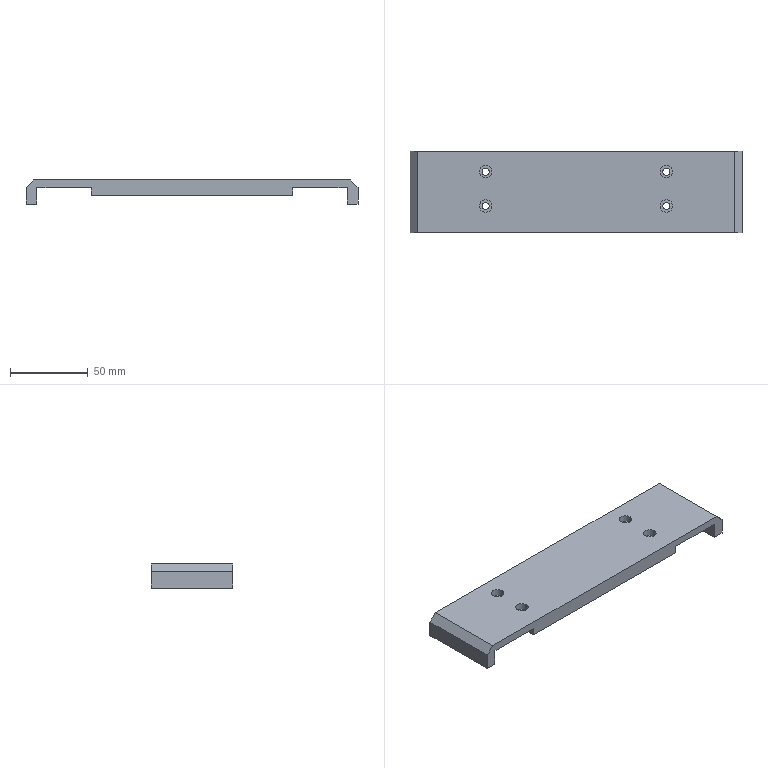Part | STEP file | (PA01.001.LX020) Stop Block A | 1 solid | 36 faces | box 213 x 52 x 15.5 mm | volume 94023 mm3 | plane 20 | cylinder 16 | commonest cylinder face diameters 4.5 x8 8 x8